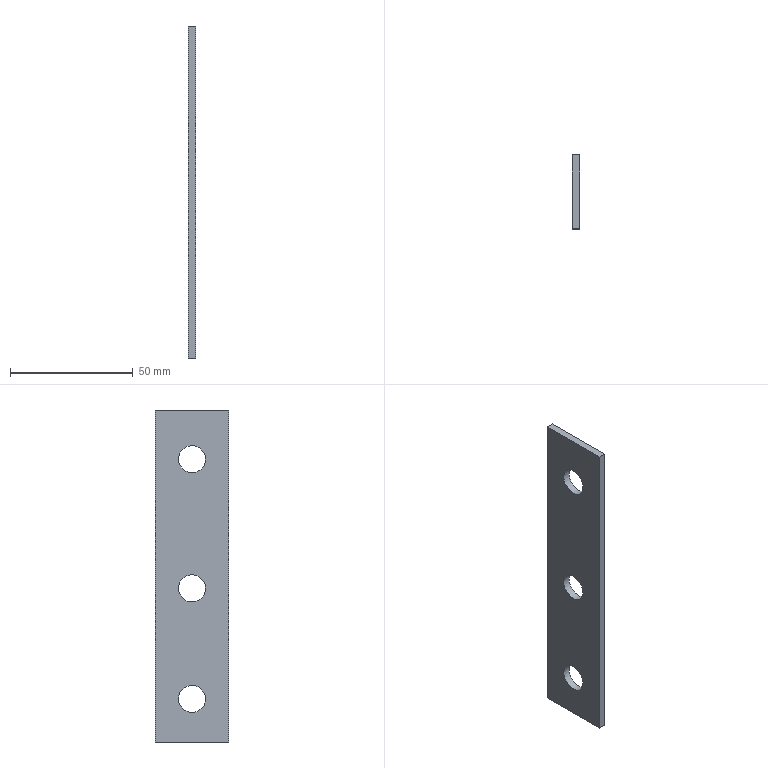Part | STEP file | SN10_016_002_SUPORTE | 1 solid | 9 faces | box 3 x 30 x 135 mm | volume 11295 mm3 | plane 6 | cylinder 3 | commonest cylinder face diameters 11 x3
STEP:
#1=CARTESIAN_POINT('',(0.,0.,0.));
#2=DIRECTION('',(0.,0.,1.));
#3=DIRECTION('',(1.,0.,0.));
#4=AXIS2_PLACEMENT_3D('',#1,#2,#3);
#5=CARTESIAN_POINT('',(5387.,-1240.173,69.863));
#6=VERTEX_POINT('',#5);
#7=CARTESIAN_POINT('',(5387.,-1245.,72.5));
#8=DIRECTION('',(1.,0.,0.));
#9=DIRECTION('',(0.,1.,0.));
#10=AXIS2_PLACEMENT_3D('',#7,#8,#9);
#11=CIRCLE('',#10,5.5);
#12=CARTESIAN_POINT('',(5386.9,-1245.,72.5));
#13=DIRECTION('',(-1.,0.,0.));
#14=DIRECTION('',(0.,0.8776,-0.4794));
#15=AXIS2_PLACEMENT_3D('',#12,#13,#14);
#16=CYLINDRICAL_SURFACE('',#15,5.5);
#17=CARTESIAN_POINT('',(12.066,-0.1));
#18=DIRECTION('',(-1.,0.));
#19=VECTOR('',#18,1.);
#20=LINE('',#17,#19);
#21=(GEOMETRIC_REPRESENTATION_CONTEXT(2)PARAMETRIC_REPRESENTATION_CONTEXT()REPRESENTATION_CONTEXT('',''));
#22=DEFINITIONAL_REPRESENTATION('',(#20),#21);
#23=PCURVE('',#16,#22);
#24=CARTESIAN_POINT('',(5387.,-1245.,92.5));
#25=DIRECTION('',(1.,0.,0.));
#26=DIRECTION('',(0.,0.,-1.));
#27=AXIS2_PLACEMENT_3D('',#24,#25,#26);
#28=PLANE('',#27);
#29=CARTESIAN_POINT('',(20.,0.));
#30=DIRECTION('',(0.,1.));
#31=AXIS2_PLACEMENT_2D('',#29,#30);
#32=CIRCLE('',#31,5.5);
#33=(GEOMETRIC_REPRESENTATION_CONTEXT(2)PARAMETRIC_REPRESENTATION_CONTEXT()REPRESENTATION_CONTEXT('',''));
#34=DEFINITIONAL_REPRESENTATION('',(#32),#33);
#35=PCURVE('',#28,#34);
#36=SURFACE_CURVE('',#11,(#23,#35),.PCURVE_S1.);
#37=EDGE_CURVE('',#6,#6,#36,.T.);
#38=ORIENTED_EDGE('',*,*,#37,.F.);
#39=CARTESIAN_POINT('',(5384.,-1240.173,69.863));
#40=VERTEX_POINT('',#39);
#41=CARTESIAN_POINT('',(5387.,-1240.173,69.863));
#42=CARTESIAN_POINT('',(5384.,-1240.173,69.863));
#43=B_SPLINE_CURVE_WITH_KNOTS('',1,(#41,#42),.UNSPECIFIED.,.F.,.F.,(2,2),(-0.1,2.9),.PIECEWISE_BEZIER_KNOTS.);
#44=CARTESIAN_POINT('',(6.283,0.));
#45=DIRECTION('',(0.,1.));
#46=VECTOR('',#45,1.);
#47=LINE('',#44,#46);
#48=(GEOMETRIC_REPRESENTATION_CONTEXT(2)PARAMETRIC_REPRESENTATION_CONTEXT()REPRESENTATION_CONTEXT('',''));
#49=DEFINITIONAL_REPRESENTATION('',(#47),#48);
#50=PCURVE('',#16,#49);
#51=CARTESIAN_POINT('',(0.,0.));
#52=DIRECTION('',(0.,1.));
#53=VECTOR('',#52,1.);
#54=LINE('',#51,#53);
#55=(GEOMETRIC_REPRESENTATION_CONTEXT(2)PARAMETRIC_REPRESENTATION_CONTEXT()REPRESENTATION_CONTEXT('',''));
#56=DEFINITIONAL_REPRESENTATION('',(#54),#55);
#57=PCURVE('',#16,#56);
#58=SEAM_CURVE('',#43,(#50,#57),.PCURVE_S1.);
#59=EDGE_CURVE('',#6,#40,#58,.T.);
#60=ORIENTED_EDGE('',*,*,#59,.T.);
#61=CARTESIAN_POINT('',(5384.,-1245.,72.5));
#62=DIRECTION('',(-1.,0.,0.));
#63=DIRECTION('',(0.,1.,0.));
#64=AXIS2_PLACEMENT_3D('',#61,#62,#63);
#65=CIRCLE('',#64,5.5);
#66=CARTESIAN_POINT('',(-0.5,2.9));
#67=DIRECTION('',(1.,0.));
#68=VECTOR('',#67,1.);
#69=LINE('',#66,#68);
#70=(GEOMETRIC_REPRESENTATION_CONTEXT(2)PARAMETRIC_REPRESENTATION_CONTEXT()REPRESENTATION_CONTEXT('',''));
#71=DEFINITIONAL_REPRESENTATION('',(#69),#70);
#72=PCURVE('',#16,#71);
#73=CARTESIAN_POINT('',(5384.,-1245.,-42.5));
#74=DIRECTION('',(-1.,0.,0.));
#75=DIRECTION('',(0.,0.,1.));
#76=AXIS2_PLACEMENT_3D('',#73,#74,#75);
#77=PLANE('',#76);
#78=CARTESIAN_POINT('',(115.,0.));
#79=DIRECTION('',(0.,1.));
#80=AXIS2_PLACEMENT_2D('',#78,#79);
#81=CIRCLE('',#80,5.5);
#82=(GEOMETRIC_REPRESENTATION_CONTEXT(2)PARAMETRIC_REPRESENTATION_CONTEXT()REPRESENTATION_CONTEXT('',''));
#83=DEFINITIONAL_REPRESENTATION('',(#81),#82);
#84=PCURVE('',#77,#83);
#85=SURFACE_CURVE('',#65,(#72,#84),.PCURVE_S1.);
#86=EDGE_CURVE('',#40,#40,#85,.T.);
#87=ORIENTED_EDGE('',*,*,#86,.F.);
#88=ORIENTED_EDGE('',*,*,#59,.F.);
#89=EDGE_LOOP('',(#38,#60,#87,#88));
#90=FACE_BOUND('',#89,.F.);
#91=ADVANCED_FACE('',(#90),#16,.F.);
#92=CARTESIAN_POINT('',(5387.,-1260.,92.5));
#93=VERTEX_POINT('',#92);
#94=CARTESIAN_POINT('',(5387.,-1230.,92.5));
#95=VERTEX_POINT('',#94);
#96=CARTESIAN_POINT('',(5387.,-1260.,92.5));
#97=DIRECTION('',(0.,1.,0.));
#98=VECTOR('',#97,1.);
#99=LINE('',#96,#98);
#100=CARTESIAN_POINT('',(0.,-15.));
#101=DIRECTION('',(0.,1.));
#102=VECTOR('',#101,1.);
#103=LINE('',#100,#102);
#104=(GEOMETRIC_REPRESENTATION_CONTEXT(2)PARAMETRIC_REPRESENTATION_CONTEXT()REPRESENTATION_CONTEXT('',''));
#105=DEFINITIONAL_REPRESENTATION('',(#103),#104);
#106=PCURVE('',#28,#105);
#107=CARTESIAN_POINT('',(5384.,-1245.,92.5));
#108=DIRECTION('',(0.,0.,1.));
#109=DIRECTION('',(1.,0.,0.));
#110=AXIS2_PLACEMENT_3D('',#107,#108,#109);
#111=PLANE('',#110);
#112=CARTESIAN_POINT('',(3.,-15.));
#113=DIRECTION('',(0.,1.));
#114=VECTOR('',#113,1.);
#115=LINE('',#112,#114);
#116=(GEOMETRIC_REPRESENTATION_CONTEXT(2)PARAMETRIC_REPRESENTATION_CONTEXT()REPRESENTATION_CONTEXT('',''));
#117=DEFINITIONAL_REPRESENTATION('',(#115),#116);
#118=PCURVE('',#111,#117);
#119=SURFACE_CURVE('',#99,(#106,#118),.PCURVE_S1.);
#120=EDGE_CURVE('',#93,#95,#119,.T.);
#121=ORIENTED_EDGE('',*,*,#120,.F.);
#122=CARTESIAN_POINT('',(5387.,-1260.,-42.5));
#123=VERTEX_POINT('',#122);
#124=CARTESIAN_POINT('',(5387.,-1260.,92.5));
#125=DIRECTION('',(0.,0.,-1.));
#126=VECTOR('',#125,1.);
#127=LINE('',#124,#126);
#128=CARTESIAN_POINT('',(0.,-15.));
#129=DIRECTION('',(1.,0.));
#130=VECTOR('',#129,1.);
#131=LINE('',#128,#130);
#132=(GEOMETRIC_REPRESENTATION_CONTEXT(2)PARAMETRIC_REPRESENTATION_CONTEXT()REPRESENTATION_CONTEXT('',''));
#133=DEFINITIONAL_REPRESENTATION('',(#131),#132);
#134=PCURVE('',#28,#133);
#135=CARTESIAN_POINT('',(5384.,-1260.,20.));
#136=DIRECTION('',(0.,1.,0.));
#137=DIRECTION('',(0.,0.,1.));
#138=AXIS2_PLACEMENT_3D('',#135,#136,#137);
#139=PLANE('',#138);
#140=CARTESIAN_POINT('',(72.5,3.));
#141=DIRECTION('',(-1.,0.));
#142=VECTOR('',#141,1.);
#143=LINE('',#140,#142);
#144=(GEOMETRIC_REPRESENTATION_CONTEXT(2)PARAMETRIC_REPRESENTATION_CONTEXT()REPRESENTATION_CONTEXT('',''));
#145=DEFINITIONAL_REPRESENTATION('',(#143),#144);
#146=PCURVE('',#139,#145);
#147=SURFACE_CURVE('',#127,(#134,#146),.PCURVE_S1.);
#148=EDGE_CURVE('',#93,#123,#147,.T.);
#149=ORIENTED_EDGE('',*,*,#148,.T.);
#150=CARTESIAN_POINT('',(5387.,-1230.,-42.5));
#151=VERTEX_POINT('',#150);
#152=CARTESIAN_POINT('',(5387.,-1260.,-42.5));
#153=DIRECTION('',(0.,1.,0.));
#154=VECTOR('',#153,1.);
#155=LINE('',#152,#154);
#156=CARTESIAN_POINT('',(135.,-15.));
#157=DIRECTION('',(0.,1.));
#158=VECTOR('',#157,1.);
#159=LINE('',#156,#158);
#160=(GEOMETRIC_REPRESENTATION_CONTEXT(2)PARAMETRIC_REPRESENTATION_CONTEXT()REPRESENTATION_CONTEXT('',''));
#161=DEFINITIONAL_REPRESENTATION('',(#159),#160);
#162=PCURVE('',#28,#161);
#163=CARTESIAN_POINT('',(5387.,-1245.,-42.5));
#164=DIRECTION('',(0.,0.,-1.));
#165=DIRECTION('',(-1.,0.,0.));
#166=AXIS2_PLACEMENT_3D('',#163,#164,#165);
#167=PLANE('',#166);
#168=CARTESIAN_POINT('',(0.,-15.));
#169=DIRECTION('',(0.,1.));
#170=VECTOR('',#169,1.);
#171=LINE('',#168,#170);
#172=(GEOMETRIC_REPRESENTATION_CONTEXT(2)PARAMETRIC_REPRESENTATION_CONTEXT()REPRESENTATION_CONTEXT('',''));
#173=DEFINITIONAL_REPRESENTATION('',(#171),#172);
#174=PCURVE('',#167,#173);
#175=SURFACE_CURVE('',#155,(#162,#174),.PCURVE_S1.);
#176=EDGE_CURVE('',#123,#151,#175,.T.);
#177=ORIENTED_EDGE('',*,*,#176,.T.);
#178=CARTESIAN_POINT('',(5387.,-1230.,92.5));
#179=DIRECTION('',(0.,0.,-1.));
#180=VECTOR('',#179,1.);
#181=LINE('',#178,#180);
#182=CARTESIAN_POINT('',(0.,15.));
#183=DIRECTION('',(1.,0.));
#184=VECTOR('',#183,1.);
#185=LINE('',#182,#184);
#186=(GEOMETRIC_REPRESENTATION_CONTEXT(2)PARAMETRIC_REPRESENTATION_CONTEXT()REPRESENTATION_CONTEXT('',''));
#187=DEFINITIONAL_REPRESENTATION('',(#185),#186);
#188=PCURVE('',#28,#187);
#189=CARTESIAN_POINT('',(5384.,-1230.,20.));
#190=DIRECTION('',(0.,1.,0.));
#191=DIRECTION('',(0.,0.,1.));
#192=AXIS2_PLACEMENT_3D('',#189,#190,#191);
#193=PLANE('',#192);
#194=CARTESIAN_POINT('',(72.5,3.));
#195=DIRECTION('',(-1.,0.));
#196=VECTOR('',#195,1.);
#197=LINE('',#194,#196);
#198=(GEOMETRIC_REPRESENTATION_CONTEXT(2)PARAMETRIC_REPRESENTATION_CONTEXT()REPRESENTATION_CONTEXT('',''));
#199=DEFINITIONAL_REPRESENTATION('',(#197),#198);
#200=PCURVE('',#193,#199);
#201=SURFACE_CURVE('',#181,(#188,#200),.PCURVE_S1.);
#202=EDGE_CURVE('',#95,#151,#201,.T.);
#203=ORIENTED_EDGE('',*,*,#202,.F.);
#204=EDGE_LOOP('',(#121,#149,#177,#203));
#205=FACE_BOUND('',#204,.T.);
#206=ORIENTED_EDGE('',*,*,#37,.F.);
#207=EDGE_LOOP('',(#206));
#208=FACE_BOUND('',#207,.T.);
#209=CARTESIAN_POINT('',(5387.,-1240.173,-27.637));
#210=VERTEX_POINT('',#209);
#211=CARTESIAN_POINT('',(5387.,-1245.,-25.));
#212=DIRECTION('',(1.,0.,0.));
#213=DIRECTION('',(0.,1.,0.));
#214=AXIS2_PLACEMENT_3D('',#211,#212,#213);
#215=CIRCLE('',#214,5.5);
#216=CARTESIAN_POINT('',(117.5,0.));
#217=DIRECTION('',(0.,1.));
#218=AXIS2_PLACEMENT_2D('',#216,#217);
#219=CIRCLE('',#218,5.5);
#220=(GEOMETRIC_REPRESENTATION_CONTEXT(2)PARAMETRIC_REPRESENTATION_CONTEXT()REPRESENTATION_CONTEXT('',''));
#221=DEFINITIONAL_REPRESENTATION('',(#219),#220);
#222=PCURVE('',#28,#221);
#223=CARTESIAN_POINT('',(5386.9,-1245.,-25.));
#224=DIRECTION('',(-1.,0.,0.));
#225=DIRECTION('',(0.,0.8776,-0.4794));
#226=AXIS2_PLACEMENT_3D('',#223,#224,#225);
#227=CYLINDRICAL_SURFACE('',#226,5.5);
#228=CARTESIAN_POINT('',(12.066,-0.1));
#229=DIRECTION('',(-1.,0.));
#230=VECTOR('',#229,1.);
#231=LINE('',#228,#230);
#232=(GEOMETRIC_REPRESENTATION_CONTEXT(2)PARAMETRIC_REPRESENTATION_CONTEXT()REPRESENTATION_CONTEXT('',''));
#233=DEFINITIONAL_REPRESENTATION('',(#231),#232);
#234=PCURVE('',#227,#233);
#235=SURFACE_CURVE('',#215,(#222,#234),.PCURVE_S1.);
#236=EDGE_CURVE('',#210,#210,#235,.T.);
#237=ORIENTED_EDGE('',*,*,#236,.F.);
#238=EDGE_LOOP('',(#237));
#239=FACE_BOUND('',#238,.T.);
#240=CARTESIAN_POINT('',(5387.,-1240.173,17.363));
#241=VERTEX_POINT('',#240);
#242=CARTESIAN_POINT('',(5387.,-1245.,20.));
#243=DIRECTION('',(1.,0.,0.));
#244=DIRECTION('',(0.,1.,0.));
#245=AXIS2_PLACEMENT_3D('',#242,#243,#244);
#246=CIRCLE('',#245,5.5);
#247=CARTESIAN_POINT('',(72.5,0.));
#248=DIRECTION('',(0.,1.));
#249=AXIS2_PLACEMENT_2D('',#247,#248);
#250=CIRCLE('',#249,5.5);
#251=(GEOMETRIC_REPRESENTATION_CONTEXT(2)PARAMETRIC_REPRESENTATION_CONTEXT()REPRESENTATION_CONTEXT('',''));
#252=DEFINITIONAL_REPRESENTATION('',(#250),#251);
#253=PCURVE('',#28,#252);
#254=CARTESIAN_POINT('',(5386.9,-1245.,20.));
#255=DIRECTION('',(-1.,0.,0.));
#256=DIRECTION('',(0.,0.8776,-0.4794));
#257=AXIS2_PLACEMENT_3D('',#254,#255,#256);
#258=CYLINDRICAL_SURFACE('',#257,5.5);
#259=CARTESIAN_POINT('',(12.066,-0.1));
#260=DIRECTION('',(-1.,0.));
#261=VECTOR('',#260,1.);
#262=LINE('',#259,#261);
#263=(GEOMETRIC_REPRESENTATION_CONTEXT(2)PARAMETRIC_REPRESENTATION_CONTEXT()REPRESENTATION_CONTEXT('',''));
#264=DEFINITIONAL_REPRESENTATION('',(#262),#263);
#265=PCURVE('',#258,#264);
#266=SURFACE_CURVE('',#246,(#253,#265),.PCURVE_S1.);
#267=EDGE_CURVE('',#241,#241,#266,.T.);
#268=ORIENTED_EDGE('',*,*,#267,.F.);
#269=EDGE_LOOP('',(#268));
#270=FACE_BOUND('',#269,.T.);
#271=ADVANCED_FACE('',(#205,#208,#239,#270),#28,.T.);
#272=CARTESIAN_POINT('',(5384.,-1260.,-42.5));
#273=VERTEX_POINT('',#272);
#274=CARTESIAN_POINT('',(5384.,-1230.,-42.5));
#275=VERTEX_POINT('',#274);
#276=CARTESIAN_POINT('',(5384.,-1260.,-42.5));
#277=DIRECTION('',(0.,1.,0.));
#278=VECTOR('',#277,1.);
#279=LINE('',#276,#278);
#280=CARTESIAN_POINT('',(0.,-15.));
#281=DIRECTION('',(0.,1.));
#282=VECTOR('',#281,1.);
#283=LINE('',#280,#282);
#284=(GEOMETRIC_REPRESENTATION_CONTEXT(2)PARAMETRIC_REPRESENTATION_CONTEXT()REPRESENTATION_CONTEXT('',''));
#285=DEFINITIONAL_REPRESENTATION('',(#283),#284);
#286=PCURVE('',#77,#285);
#287=CARTESIAN_POINT('',(3.,-15.));
#288=DIRECTION('',(0.,1.));
#289=VECTOR('',#288,1.);
#290=LINE('',#287,#289);
#291=(GEOMETRIC_REPRESENTATION_CONTEXT(2)PARAMETRIC_REPRESENTATION_CONTEXT()REPRESENTATION_CONTEXT('',''));
#292=DEFINITIONAL_REPRESENTATION('',(#290),#291);
#293=PCURVE('',#167,#292);
#294=SURFACE_CURVE('',#279,(#286,#293),.PCURVE_S1.);
#295=EDGE_CURVE('',#273,#275,#294,.T.);
#296=ORIENTED_EDGE('',*,*,#295,.F.);
#297=CARTESIAN_POINT('',(5384.,-1260.,92.5));
#298=VERTEX_POINT('',#297);
#299=CARTESIAN_POINT('',(5384.,-1260.,-42.5));
#300=DIRECTION('',(0.,0.,1.));
#301=VECTOR('',#300,1.);
#302=LINE('',#299,#301);
#303=CARTESIAN_POINT('',(0.,-15.));
#304=DIRECTION('',(1.,0.));
#305=VECTOR('',#304,1.);
#306=LINE('',#303,#305);
#307=(GEOMETRIC_REPRESENTATION_CONTEXT(2)PARAMETRIC_REPRESENTATION_CONTEXT()REPRESENTATION_CONTEXT('',''));
#308=DEFINITIONAL_REPRESENTATION('',(#306),#307);
#309=PCURVE('',#77,#308);
#310=CARTESIAN_POINT('',(-62.5,0.));
#311=DIRECTION('',(1.,0.));
#312=VECTOR('',#311,1.);
#313=LINE('',#310,#312);
#314=(GEOMETRIC_REPRESENTATION_CONTEXT(2)PARAMETRIC_REPRESENTATION_CONTEXT()REPRESENTATION_CONTEXT('',''));
#315=DEFINITIONAL_REPRESENTATION('',(#313),#314);
#316=PCURVE('',#139,#315);
#317=SURFACE_CURVE('',#302,(#309,#316),.PCURVE_S1.);
#318=EDGE_CURVE('',#273,#298,#317,.T.);
#319=ORIENTED_EDGE('',*,*,#318,.T.);
#320=CARTESIAN_POINT('',(5384.,-1230.,92.5));
#321=VERTEX_POINT('',#320);
#322=CARTESIAN_POINT('',(5384.,-1260.,92.5));
#323=DIRECTION('',(0.,1.,0.));
#324=VECTOR('',#323,1.);
#325=LINE('',#322,#324);
#326=CARTESIAN_POINT('',(135.,-15.));
#327=DIRECTION('',(0.,1.));
#328=VECTOR('',#327,1.);
#329=LINE('',#326,#328);
#330=(GEOMETRIC_REPRESENTATION_CONTEXT(2)PARAMETRIC_REPRESENTATION_CONTEXT()REPRESENTATION_CONTEXT('',''));
#331=DEFINITIONAL_REPRESENTATION('',(#329),#330);
#332=PCURVE('',#77,#331);
#333=CARTESIAN_POINT('',(0.,-15.));
#334=DIRECTION('',(0.,1.));
#335=VECTOR('',#334,1.);
#336=LINE('',#333,#335);
#337=(GEOMETRIC_REPRESENTATION_CONTEXT(2)PARAMETRIC_REPRESENTATION_CONTEXT()REPRESENTATION_CONTEXT('',''));
#338=DEFINITIONAL_REPRESENTATION('',(#336),#337);
#339=PCURVE('',#111,#338);
#340=SURFACE_CURVE('',#325,(#332,#339),.PCURVE_S1.);
#341=EDGE_CURVE('',#298,#321,#340,.T.);
#342=ORIENTED_EDGE('',*,*,#341,.T.);
#343=CARTESIAN_POINT('',(5384.,-1230.,-42.5));
#344=DIRECTION('',(0.,0.,1.));
#345=VECTOR('',#344,1.);
#346=LINE('',#343,#345);
#347=CARTESIAN_POINT('',(0.,15.));
#348=DIRECTION('',(1.,0.));
#349=VECTOR('',#348,1.);
#350=LINE('',#347,#349);
#351=(GEOMETRIC_REPRESENTATION_CONTEXT(2)PARAMETRIC_REPRESENTATION_CONTEXT()REPRESENTATION_CONTEXT('',''));
#352=DEFINITIONAL_REPRESENTATION('',(#350),#351);
#353=PCURVE('',#77,#352);
#354=CARTESIAN_POINT('',(-62.5,0.));
#355=DIRECTION('',(1.,0.));
#356=VECTOR('',#355,1.);
#357=LINE('',#354,#356);
#358=(GEOMETRIC_REPRESENTATION_CONTEXT(2)PARAMETRIC_REPRESENTATION_CONTEXT()REPRESENTATION_CONTEXT('',''));
#359=DEFINITIONAL_REPRESENTATION('',(#357),#358);
#360=PCURVE('',#193,#359);
#361=SURFACE_CURVE('',#346,(#353,#360),.PCURVE_S1.);
#362=EDGE_CURVE('',#275,#321,#361,.T.);
#363=ORIENTED_EDGE('',*,*,#362,.F.);
#364=EDGE_LOOP('',(#296,#319,#342,#363));
#365=FACE_BOUND('',#364,.T.);
#366=ORIENTED_EDGE('',*,*,#86,.F.);
#367=EDGE_LOOP('',(#366));
#368=FACE_BOUND('',#367,.T.);
#369=CARTESIAN_POINT('',(5384.,-1240.173,-27.637));
#370=VERTEX_POINT('',#369);
#371=CARTESIAN_POINT('',(5384.,-1245.,-25.));
#372=DIRECTION('',(-1.,0.,0.));
#373=DIRECTION('',(0.,1.,0.));
#374=AXIS2_PLACEMENT_3D('',#371,#372,#373);
#375=CIRCLE('',#374,5.5);
#376=CARTESIAN_POINT('',(17.5,0.));
#377=DIRECTION('',(0.,1.));
#378=AXIS2_PLACEMENT_2D('',#376,#377);
#379=CIRCLE('',#378,5.5);
#380=(GEOMETRIC_REPRESENTATION_CONTEXT(2)PARAMETRIC_REPRESENTATION_CONTEXT()REPRESENTATION_CONTEXT('',''));
#381=DEFINITIONAL_REPRESENTATION('',(#379),#380);
#382=PCURVE('',#77,#381);
#383=CARTESIAN_POINT('',(-0.5,2.9));
#384=DIRECTION('',(1.,0.));
#385=VECTOR('',#384,1.);
#386=LINE('',#383,#385);
#387=(GEOMETRIC_REPRESENTATION_CONTEXT(2)PARAMETRIC_REPRESENTATION_CONTEXT()REPRESENTATION_CONTEXT('',''));
#388=DEFINITIONAL_REPRESENTATION('',(#386),#387);
#389=PCURVE('',#227,#388);
#390=SURFACE_CURVE('',#375,(#382,#389),.PCURVE_S1.);
#391=EDGE_CURVE('',#370,#370,#390,.T.);
#392=ORIENTED_EDGE('',*,*,#391,.F.);
#393=EDGE_LOOP('',(#392));
#394=FACE_BOUND('',#393,.T.);
#395=CARTESIAN_POINT('',(5384.,-1240.173,17.363));
#396=VERTEX_POINT('',#395);
#397=CARTESIAN_POINT('',(5384.,-1245.,20.));
#398=DIRECTION('',(-1.,0.,0.));
#399=DIRECTION('',(0.,1.,0.));
#400=AXIS2_PLACEMENT_3D('',#397,#398,#399);
#401=CIRCLE('',#400,5.5);
#402=CARTESIAN_POINT('',(62.5,0.));
#403=DIRECTION('',(0.,1.));
#404=AXIS2_PLACEMENT_2D('',#402,#403);
#405=CIRCLE('',#404,5.5);
#406=(GEOMETRIC_REPRESENTATION_CONTEXT(2)PARAMETRIC_REPRESENTATION_CONTEXT()REPRESENTATION_CONTEXT('',''));
#407=DEFINITIONAL_REPRESENTATION('',(#405),#406);
#408=PCURVE('',#77,#407);
#409=CARTESIAN_POINT('',(-0.5,2.9));
#410=DIRECTION('',(1.,0.));
#411=VECTOR('',#410,1.);
#412=LINE('',#409,#411);
#413=(GEOMETRIC_REPRESENTATION_CONTEXT(2)PARAMETRIC_REPRESENTATION_CONTEXT()REPRESENTATION_CONTEXT('',''));
#414=DEFINITIONAL_REPRESENTATION('',(#412),#413);
#415=PCURVE('',#258,#414);
#416=SURFACE_CURVE('',#401,(#408,#415),.PCURVE_S1.);
#417=EDGE_CURVE('',#396,#396,#416,.T.);
#418=ORIENTED_EDGE('',*,*,#417,.F.);
#419=EDGE_LOOP('',(#418));
#420=FACE_BOUND('',#419,.T.);
#421=ADVANCED_FACE('',(#365,#368,#394,#420),#77,.T.);
#422=CARTESIAN_POINT('',(5387.,-1260.,-42.5));
#423=DIRECTION('',(-1.,0.,0.));
#424=VECTOR('',#423,1.);
#425=LINE('',#422,#424);
#426=CARTESIAN_POINT('',(-62.5,3.));
#427=DIRECTION('',(0.,-1.));
#428=VECTOR('',#427,1.);
#429=LINE('',#426,#428);
#430=(GEOMETRIC_REPRESENTATION_CONTEXT(2)PARAMETRIC_REPRESENTATION_CONTEXT()REPRESENTATION_CONTEXT('',''));
#431=DEFINITIONAL_REPRESENTATION('',(#429),#430);
#432=PCURVE('',#139,#431);
#433=CARTESIAN_POINT('',(0.,-15.));
#434=DIRECTION('',(1.,0.));
#435=VECTOR('',#434,1.);
#436=LINE('',#433,#435);
#437=(GEOMETRIC_REPRESENTATION_CONTEXT(2)PARAMETRIC_REPRESENTATION_CONTEXT()REPRESENTATION_CONTEXT('',''));
#438=DEFINITIONAL_REPRESENTATION('',(#436),#437);
#439=PCURVE('',#167,#438);
#440=SURFACE_CURVE('',#425,(#432,#439),.PCURVE_S1.);
#441=EDGE_CURVE('',#123,#273,#440,.T.);
#442=ORIENTED_EDGE('',*,*,#441,.F.);
#443=ORIENTED_EDGE('',*,*,#148,.F.);
#444=CARTESIAN_POINT('',(5384.,-1260.,92.5));
#445=DIRECTION('',(1.,0.,0.));
#446=VECTOR('',#445,1.);
#447=LINE('',#444,#446);
#448=CARTESIAN_POINT('',(72.5,0.));
#449=DIRECTION('',(0.,1.));
#450=VECTOR('',#449,1.);
#451=LINE('',#448,#450);
#452=(GEOMETRIC_REPRESENTATION_CONTEXT(2)PARAMETRIC_REPRESENTATION_CONTEXT()REPRESENTATION_CONTEXT('',''));
#453=DEFINITIONAL_REPRESENTATION('',(#451),#452);
#454=PCURVE('',#139,#453);
#455=CARTESIAN_POINT('',(0.,-15.));
#456=DIRECTION('',(1.,0.));
#457=VECTOR('',#456,1.);
#458=LINE('',#455,#457);
#459=(GEOMETRIC_REPRESENTATION_CONTEXT(2)PARAMETRIC_REPRESENTATION_CONTEXT()REPRESENTATION_CONTEXT('',''));
#460=DEFINITIONAL_REPRESENTATION('',(#458),#459);
#461=PCURVE('',#111,#460);
#462=SURFACE_CURVE('',#447,(#454,#461),.PCURVE_S1.);
#463=EDGE_CURVE('',#298,#93,#462,.T.);
#464=ORIENTED_EDGE('',*,*,#463,.F.);
#465=ORIENTED_EDGE('',*,*,#318,.F.);
#466=EDGE_LOOP('',(#442,#443,#464,#465));
#467=FACE_BOUND('',#466,.T.);
#468=ADVANCED_FACE('',(#467),#139,.F.);
#469=ORIENTED_EDGE('',*,*,#176,.F.);
#470=ORIENTED_EDGE('',*,*,#441,.T.);
#471=ORIENTED_EDGE('',*,*,#295,.T.);
#472=CARTESIAN_POINT('',(5387.,-1230.,-42.5));
#473=DIRECTION('',(-1.,0.,0.));
#474=VECTOR('',#473,1.);
#475=LINE('',#472,#474);
#476=CARTESIAN_POINT('',(0.,15.));
#477=DIRECTION('',(1.,0.));
#478=VECTOR('',#477,1.);
#479=LINE('',#476,#478);
#480=(GEOMETRIC_REPRESENTATION_CONTEXT(2)PARAMETRIC_REPRESENTATION_CONTEXT()REPRESENTATION_CONTEXT('',''));
#481=DEFINITIONAL_REPRESENTATION('',(#479),#480);
#482=PCURVE('',#167,#481);
#483=CARTESIAN_POINT('',(-62.5,3.));
#484=DIRECTION('',(0.,-1.));
#485=VECTOR('',#484,1.);
#486=LINE('',#483,#485);
#487=(GEOMETRIC_REPRESENTATION_CONTEXT(2)PARAMETRIC_REPRESENTATION_CONTEXT()REPRESENTATION_CONTEXT('',''));
#488=DEFINITIONAL_REPRESENTATION('',(#486),#487);
#489=PCURVE('',#193,#488);
#490=SURFACE_CURVE('',#475,(#482,#489),.PCURVE_S1.);
#491=EDGE_CURVE('',#151,#275,#490,.T.);
#492=ORIENTED_EDGE('',*,*,#491,.F.);
#493=EDGE_LOOP('',(#469,#470,#471,#492));
#494=FACE_BOUND('',#493,.T.);
#495=ADVANCED_FACE('',(#494),#167,.T.);
#496=ORIENTED_EDGE('',*,*,#267,.F.);
#497=CARTESIAN_POINT('',(5387.,-1240.173,17.363));
#498=CARTESIAN_POINT('',(5384.,-1240.173,17.363));
#499=B_SPLINE_CURVE_WITH_KNOTS('',1,(#497,#498),.UNSPECIFIED.,.F.,.F.,(2,2),(-0.1,2.9),.PIECEWISE_BEZIER_KNOTS.);
#500=CARTESIAN_POINT('',(6.283,0.));
#501=DIRECTION('',(0.,1.));
#502=VECTOR('',#501,1.);
#503=LINE('',#500,#502);
#504=(GEOMETRIC_REPRESENTATION_CONTEXT(2)PARAMETRIC_REPRESENTATION_CONTEXT()REPRESENTATION_CONTEXT('',''));
#505=DEFINITIONAL_REPRESENTATION('',(#503),#504);
#506=PCURVE('',#258,#505);
#507=CARTESIAN_POINT('',(0.,0.));
#508=DIRECTION('',(0.,1.));
#509=VECTOR('',#508,1.);
#510=LINE('',#507,#509);
#511=(GEOMETRIC_REPRESENTATION_CONTEXT(2)PARAMETRIC_REPRESENTATION_CONTEXT()REPRESENTATION_CONTEXT('',''));
#512=DEFINITIONAL_REPRESENTATION('',(#510),#511);
#513=PCURVE('',#258,#512);
#514=SEAM_CURVE('',#499,(#506,#513),.PCURVE_S1.);
#515=EDGE_CURVE('',#241,#396,#514,.T.);
#516=ORIENTED_EDGE('',*,*,#515,.T.);
#517=ORIENTED_EDGE('',*,*,#417,.F.);
#518=ORIENTED_EDGE('',*,*,#515,.F.);
#519=EDGE_LOOP('',(#496,#516,#517,#518));
#520=FACE_BOUND('',#519,.F.);
#521=ADVANCED_FACE('',(#520),#258,.F.);
#522=ORIENTED_EDGE('',*,*,#236,.F.);
#523=CARTESIAN_POINT('',(5387.,-1240.173,-27.637));
#524=CARTESIAN_POINT('',(5384.,-1240.173,-27.637));
#525=B_SPLINE_CURVE_WITH_KNOTS('',1,(#523,#524),.UNSPECIFIED.,.F.,.F.,(2,2),(-0.1,2.9),.PIECEWISE_BEZIER_KNOTS.);
#526=CARTESIAN_POINT('',(6.283,0.));
#527=DIRECTION('',(0.,1.));
#528=VECTOR('',#527,1.);
#529=LINE('',#526,#528);
#530=(GEOMETRIC_REPRESENTATION_CONTEXT(2)PARAMETRIC_REPRESENTATION_CONTEXT()REPRESENTATION_CONTEXT('',''));
#531=DEFINITIONAL_REPRESENTATION('',(#529),#530);
#532=PCURVE('',#227,#531);
#533=CARTESIAN_POINT('',(0.,0.));
#534=DIRECTION('',(0.,1.));
#535=VECTOR('',#534,1.);
#536=LINE('',#533,#535);
#537=(GEOMETRIC_REPRESENTATION_CONTEXT(2)PARAMETRIC_REPRESENTATION_CONTEXT()REPRESENTATION_CONTEXT('',''));
#538=DEFINITIONAL_REPRESENTATION('',(#536),#537);
#539=PCURVE('',#227,#538);
#540=SEAM_CURVE('',#525,(#532,#539),.PCURVE_S1.);
#541=EDGE_CURVE('',#210,#370,#540,.T.);
#542=ORIENTED_EDGE('',*,*,#541,.T.);
#543=ORIENTED_EDGE('',*,*,#391,.F.);
#544=ORIENTED_EDGE('',*,*,#541,.F.);
#545=EDGE_LOOP('',(#522,#542,#543,#544));
#546=FACE_BOUND('',#545,.F.);
#547=ADVANCED_FACE('',(#546),#227,.F.);
#548=ORIENTED_EDGE('',*,*,#362,.T.);
#549=CARTESIAN_POINT('',(5384.,-1230.,92.5));
#550=DIRECTION('',(1.,0.,0.));
#551=VECTOR('',#550,1.);
#552=LINE('',#549,#551);
#553=CARTESIAN_POINT('',(72.5,0.));
#554=DIRECTION('',(0.,1.));
#555=VECTOR('',#554,1.);
#556=LINE('',#553,#555);
#557=(GEOMETRIC_REPRESENTATION_CONTEXT(2)PARAMETRIC_REPRESENTATION_CONTEXT()REPRESENTATION_CONTEXT('',''));
#558=DEFINITIONAL_REPRESENTATION('',(#556),#557);
#559=PCURVE('',#193,#558);
#560=CARTESIAN_POINT('',(0.,15.));
#561=DIRECTION('',(1.,0.));
#562=VECTOR('',#561,1.);
#563=LINE('',#560,#562);
#564=(GEOMETRIC_REPRESENTATION_CONTEXT(2)PARAMETRIC_REPRESENTATION_CONTEXT()REPRESENTATION_CONTEXT('',''));
#565=DEFINITIONAL_REPRESENTATION('',(#563),#564);
#566=PCURVE('',#111,#565);
#567=SURFACE_CURVE('',#552,(#559,#566),.PCURVE_S1.);
#568=EDGE_CURVE('',#321,#95,#567,.T.);
#569=ORIENTED_EDGE('',*,*,#568,.T.);
#570=ORIENTED_EDGE('',*,*,#202,.T.);
#571=ORIENTED_EDGE('',*,*,#491,.T.);
#572=EDGE_LOOP('',(#548,#569,#570,#571));
#573=FACE_BOUND('',#572,.T.);
#574=ADVANCED_FACE('',(#573),#193,.T.);
#575=ORIENTED_EDGE('',*,*,#341,.F.);
#576=ORIENTED_EDGE('',*,*,#463,.T.);
#577=ORIENTED_EDGE('',*,*,#120,.T.);
#578=ORIENTED_EDGE('',*,*,#568,.F.);
#579=EDGE_LOOP('',(#575,#576,#577,#578));
#580=FACE_BOUND('',#579,.T.);
#581=ADVANCED_FACE('',(#580),#111,.T.);
#582=CLOSED_SHELL('',(#91,#271,#421,#468,#495,#521,#547,#574,#581));
#583=MANIFOLD_SOLID_BREP('',#582);
#584=(LENGTH_UNIT()NAMED_UNIT(*)SI_UNIT(.MILLI.,.METRE.));
#585=UNCERTAINTY_MEASURE_WITH_UNIT(LENGTH_MEASURE(0.000002),#584,'','');
#586=(NAMED_UNIT(*)PLANE_ANGLE_UNIT()SI_UNIT($,.RADIAN.));
#587=(NAMED_UNIT(*)SI_UNIT($,.STERADIAN.)SOLID_ANGLE_UNIT());
#588=(GEOMETRIC_REPRESENTATION_CONTEXT(3)GLOBAL_UNCERTAINTY_ASSIGNED_CONTEXT((#585))GLOBAL_UNIT_ASSIGNED_CONTEXT((#584,#586,#587))REPRESENTATION_CONTEXT('',''));
#589=ADVANCED_BREP_SHAPE_REPRESENTATION('',(#4,#583),#588);